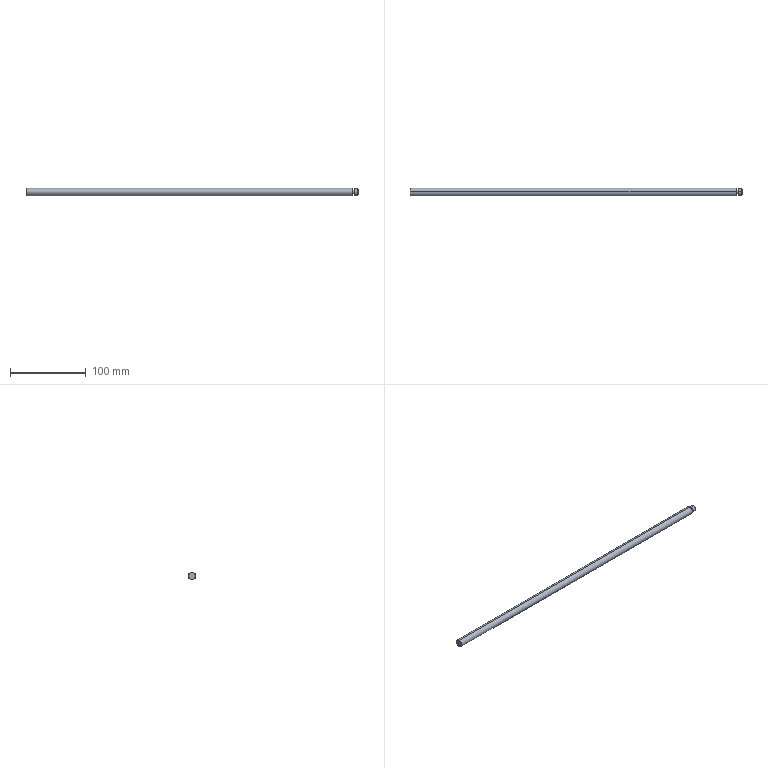Part | SolidWorks | features ICE 2, Chamfer 1, Extrusion 1 | 1 solid | 16 faces | box 437 x 10 x 10 mm | volume 34052 mm3 | cone 6 | cylinder 6 | plane 4 | commonest cylinder face diameters 5 x2 8 x2 10 x2
STEP:
#1=CARTESIAN_POINT('',(215.,0.,-4.5));
#2=VERTEX_POINT('',#1);
#3=CARTESIAN_POINT('',(215.,0.,4.5));
#4=VERTEX_POINT('',#3);
#5=CARTESIAN_POINT('',(215.,0.,0.));
#6=DIRECTION('',(1.,0.,0.));
#7=DIRECTION('',(0.,0.,-1.));
#8=AXIS2_PLACEMENT_3D('',#5,#6,#7);
#9=CIRCLE('',#8,4.5);
#10=EDGE_CURVE('',#2,#4,#9,.T.);
#11=ORIENTED_EDGE('',*,*,#10,.F.);
#12=CARTESIAN_POINT('',(214.5,0.,-5.));
#13=VERTEX_POINT('',#12);
#14=CARTESIAN_POINT('',(215.,0.,-4.5));
#15=DIRECTION('',(-0.7071,0.,-0.7071));
#16=VECTOR('',#15,1000.);
#17=LINE('',#14,#16);
#18=EDGE_CURVE('',#2,#13,#17,.T.);
#19=ORIENTED_EDGE('',*,*,#18,.T.);
#20=CARTESIAN_POINT('',(214.5,0.,5.));
#21=VERTEX_POINT('',#20);
#22=CARTESIAN_POINT('',(214.5,0.,0.));
#23=DIRECTION('',(-1.,0.,0.));
#24=DIRECTION('',(0.,0.,-1.));
#25=AXIS2_PLACEMENT_3D('',#22,#23,#24);
#26=CIRCLE('',#25,5.);
#27=EDGE_CURVE('',#21,#13,#26,.T.);
#28=ORIENTED_EDGE('',*,*,#27,.F.);
#29=CARTESIAN_POINT('',(215.,0.,4.5));
#30=DIRECTION('',(-0.7071,0.,0.7071));
#31=VECTOR('',#30,1000.);
#32=LINE('',#29,#31);
#33=EDGE_CURVE('',#4,#21,#32,.T.);
#34=ORIENTED_EDGE('',*,*,#33,.F.);
#35=EDGE_LOOP('',(#11,#19,#28,#34));
#36=FACE_OUTER_BOUND('',#35,.T.);
#37=CARTESIAN_POINT('',(215.,0.,0.));
#38=DIRECTION('',(-1.,0.,0.));
#39=DIRECTION('',(0.,0.,1.));
#40=AXIS2_PLACEMENT_3D('',#37,#38,#39);
#41=CONICAL_SURFACE('',#40,4.5,0.7854);
#42=ADVANCED_FACE('',(#36),#41,.T.);
#43=CARTESIAN_POINT('',(-215.,0.,4.5));
#44=VERTEX_POINT('',#43);
#45=CARTESIAN_POINT('',(-215.,0.,-4.5));
#46=VERTEX_POINT('',#45);
#47=CARTESIAN_POINT('',(-215.,0.,0.));
#48=DIRECTION('',(-1.,0.,0.));
#49=DIRECTION('',(0.,0.,-1.));
#50=AXIS2_PLACEMENT_3D('',#47,#48,#49);
#51=CIRCLE('',#50,4.5);
#52=EDGE_CURVE('',#44,#46,#51,.T.);
#53=ORIENTED_EDGE('',*,*,#52,.F.);
#54=CARTESIAN_POINT('',(-214.5,0.,5.));
#55=VERTEX_POINT('',#54);
#56=CARTESIAN_POINT('',(-214.5,0.,5.));
#57=DIRECTION('',(0.7071,0.,0.7071));
#58=VECTOR('',#57,1000.);
#59=LINE('',#56,#58);
#60=EDGE_CURVE('',#44,#55,#59,.T.);
#61=ORIENTED_EDGE('',*,*,#60,.T.);
#62=CARTESIAN_POINT('',(-214.5,0.,-5.));
#63=VERTEX_POINT('',#62);
#64=CARTESIAN_POINT('',(-214.5,0.,0.));
#65=DIRECTION('',(1.,0.,0.));
#66=DIRECTION('',(0.,0.,-1.));
#67=AXIS2_PLACEMENT_3D('',#64,#65,#66);
#68=CIRCLE('',#67,5.);
#69=EDGE_CURVE('',#63,#55,#68,.T.);
#70=ORIENTED_EDGE('',*,*,#69,.F.);
#71=CARTESIAN_POINT('',(-214.5,0.,-5.));
#72=DIRECTION('',(0.7071,0.,-0.7071));
#73=VECTOR('',#72,1000.);
#74=LINE('',#71,#73);
#75=EDGE_CURVE('',#46,#63,#74,.T.);
#76=ORIENTED_EDGE('',*,*,#75,.F.);
#77=EDGE_LOOP('',(#53,#61,#70,#76));
#78=FACE_OUTER_BOUND('',#77,.T.);
#79=CARTESIAN_POINT('',(-214.5,0.,0.));
#80=DIRECTION('',(1.,0.,0.));
#81=DIRECTION('',(0.,0.,-1.));
#82=AXIS2_PLACEMENT_3D('',#79,#80,#81);
#83=CONICAL_SURFACE('',#82,5.,0.7854);
#84=ADVANCED_FACE('',(#78),#83,.T.);
#85=CARTESIAN_POINT('',(222.,0.,-3.5));
#86=VERTEX_POINT('',#85);
#87=CARTESIAN_POINT('',(222.,0.,3.5));
#88=VERTEX_POINT('',#87);
#89=CARTESIAN_POINT('',(222.,0.,0.));
#90=DIRECTION('',(1.,0.,0.));
#91=DIRECTION('',(0.,0.,-1.));
#92=AXIS2_PLACEMENT_3D('',#89,#90,#91);
#93=CIRCLE('',#92,3.5);
#94=EDGE_CURVE('',#86,#88,#93,.T.);
#95=ORIENTED_EDGE('',*,*,#94,.F.);
#96=CARTESIAN_POINT('',(221.5,0.,-4.));
#97=VERTEX_POINT('',#96);
#98=CARTESIAN_POINT('',(222.,0.,-3.5));
#99=DIRECTION('',(-0.7071,0.,-0.7071));
#100=VECTOR('',#99,1000.);
#101=LINE('',#98,#100);
#102=EDGE_CURVE('',#86,#97,#101,.T.);
#103=ORIENTED_EDGE('',*,*,#102,.T.);
#104=CARTESIAN_POINT('',(221.5,0.,4.));
#105=VERTEX_POINT('',#104);
#106=CARTESIAN_POINT('',(221.5,0.,0.));
#107=DIRECTION('',(-1.,0.,0.));
#108=DIRECTION('',(0.,0.,-1.));
#109=AXIS2_PLACEMENT_3D('',#106,#107,#108);
#110=CIRCLE('',#109,4.);
#111=EDGE_CURVE('',#105,#97,#110,.T.);
#112=ORIENTED_EDGE('',*,*,#111,.F.);
#113=CARTESIAN_POINT('',(222.,0.,3.5));
#114=DIRECTION('',(-0.7071,0.,0.7071));
#115=VECTOR('',#114,1000.);
#116=LINE('',#113,#115);
#117=EDGE_CURVE('',#88,#105,#116,.T.);
#118=ORIENTED_EDGE('',*,*,#117,.F.);
#119=EDGE_LOOP('',(#95,#103,#112,#118));
#120=FACE_OUTER_BOUND('',#119,.T.);
#121=CARTESIAN_POINT('',(222.,0.,0.));
#122=DIRECTION('',(-1.,0.,0.));
#123=DIRECTION('',(0.,0.,1.));
#124=AXIS2_PLACEMENT_3D('',#121,#122,#123);
#125=CONICAL_SURFACE('',#124,3.5,0.7854);
#126=ADVANCED_FACE('',(#120),#125,.T.);
#127=ORIENTED_EDGE('',*,*,#111,.T.);
#128=CARTESIAN_POINT('',(217.,0.,-4.));
#129=VERTEX_POINT('',#128);
#130=CARTESIAN_POINT('',(222.,0.,-4.));
#131=DIRECTION('',(-1.,0.,0.));
#132=VECTOR('',#131,1000.);
#133=LINE('',#130,#132);
#134=EDGE_CURVE('',#97,#129,#133,.T.);
#135=ORIENTED_EDGE('',*,*,#134,.T.);
#136=CARTESIAN_POINT('',(217.,0.,4.));
#137=VERTEX_POINT('',#136);
#138=CARTESIAN_POINT('',(217.,0.,0.));
#139=DIRECTION('',(1.,0.,0.));
#140=DIRECTION('',(0.,0.,-1.));
#141=AXIS2_PLACEMENT_3D('',#138,#139,#140);
#142=CIRCLE('',#141,4.);
#143=EDGE_CURVE('',#129,#137,#142,.T.);
#144=ORIENTED_EDGE('',*,*,#143,.T.);
#145=CARTESIAN_POINT('',(222.,0.,4.));
#146=DIRECTION('',(-1.,0.,0.));
#147=VECTOR('',#146,1000.);
#148=LINE('',#145,#147);
#149=EDGE_CURVE('',#105,#137,#148,.T.);
#150=ORIENTED_EDGE('',*,*,#149,.F.);
#151=EDGE_LOOP('',(#127,#135,#144,#150));
#152=FACE_OUTER_BOUND('',#151,.T.);
#153=CARTESIAN_POINT('',(222.,0.,0.));
#154=DIRECTION('',(-1.,0.,0.));
#155=DIRECTION('',(0.,0.,1.));
#156=AXIS2_PLACEMENT_3D('',#153,#154,#155);
#157=CYLINDRICAL_SURFACE('',#156,4.);
#158=ADVANCED_FACE('',(#152),#157,.T.);
#159=CARTESIAN_POINT('',(217.,0.,-2.5));
#160=VERTEX_POINT('',#159);
#161=CARTESIAN_POINT('',(217.,0.,2.5));
#162=VERTEX_POINT('',#161);
#163=CARTESIAN_POINT('',(217.,0.,0.));
#164=DIRECTION('',(1.,0.,0.));
#165=DIRECTION('',(0.,0.,-1.));
#166=AXIS2_PLACEMENT_3D('',#163,#164,#165);
#167=CIRCLE('',#166,2.5);
#168=EDGE_CURVE('',#160,#162,#167,.T.);
#169=ORIENTED_EDGE('',*,*,#168,.F.);
#170=CARTESIAN_POINT('',(215.,0.,-2.5));
#171=VERTEX_POINT('',#170);
#172=CARTESIAN_POINT('',(217.,0.,-2.5));
#173=DIRECTION('',(-1.,0.,0.));
#174=VECTOR('',#173,1000.);
#175=LINE('',#172,#174);
#176=EDGE_CURVE('',#160,#171,#175,.T.);
#177=ORIENTED_EDGE('',*,*,#176,.T.);
#178=CARTESIAN_POINT('',(215.,0.,2.5));
#179=VERTEX_POINT('',#178);
#180=CARTESIAN_POINT('',(215.,0.,0.));
#181=DIRECTION('',(1.,0.,0.));
#182=DIRECTION('',(0.,0.,-1.));
#183=AXIS2_PLACEMENT_3D('',#180,#181,#182);
#184=CIRCLE('',#183,2.5);
#185=EDGE_CURVE('',#171,#179,#184,.T.);
#186=ORIENTED_EDGE('',*,*,#185,.T.);
#187=CARTESIAN_POINT('',(217.,0.,2.5));
#188=DIRECTION('',(-1.,0.,0.));
#189=VECTOR('',#188,1000.);
#190=LINE('',#187,#189);
#191=EDGE_CURVE('',#162,#179,#190,.T.);
#192=ORIENTED_EDGE('',*,*,#191,.F.);
#193=EDGE_LOOP('',(#169,#177,#186,#192));
#194=FACE_OUTER_BOUND('',#193,.T.);
#195=CARTESIAN_POINT('',(217.,0.,0.));
#196=DIRECTION('',(-1.,0.,0.));
#197=DIRECTION('',(0.,0.,1.));
#198=AXIS2_PLACEMENT_3D('',#195,#196,#197);
#199=CYLINDRICAL_SURFACE('',#198,2.5);
#200=ADVANCED_FACE('',(#194),#199,.T.);
#201=ORIENTED_EDGE('',*,*,#27,.T.);
#202=CARTESIAN_POINT('',(215.,0.,-5.));
#203=DIRECTION('',(-1.,0.,0.));
#204=VECTOR('',#203,1000.);
#205=LINE('',#202,#204);
#206=EDGE_CURVE('',#13,#63,#205,.T.);
#207=ORIENTED_EDGE('',*,*,#206,.T.);
#208=ORIENTED_EDGE('',*,*,#69,.T.);
#209=CARTESIAN_POINT('',(215.,0.,5.));
#210=DIRECTION('',(-1.,0.,0.));
#211=VECTOR('',#210,1000.);
#212=LINE('',#209,#211);
#213=EDGE_CURVE('',#21,#55,#212,.T.);
#214=ORIENTED_EDGE('',*,*,#213,.F.);
#215=EDGE_LOOP('',(#201,#207,#208,#214));
#216=FACE_OUTER_BOUND('',#215,.T.);
#217=CARTESIAN_POINT('',(215.,0.,0.));
#218=DIRECTION('',(-1.,0.,0.));
#219=DIRECTION('',(0.,0.,1.));
#220=AXIS2_PLACEMENT_3D('',#217,#218,#219);
#221=CYLINDRICAL_SURFACE('',#220,5.);
#222=ADVANCED_FACE('',(#216),#221,.T.);
#223=CARTESIAN_POINT('',(215.,0.,0.));
#224=DIRECTION('',(1.,0.,0.));
#225=DIRECTION('',(0.,0.,-1.));
#226=AXIS2_PLACEMENT_3D('',#223,#224,#225);
#227=CIRCLE('',#226,4.5);
#228=EDGE_CURVE('',#4,#2,#227,.T.);
#229=ORIENTED_EDGE('',*,*,#228,.T.);
#230=ORIENTED_EDGE('',*,*,#10,.T.);
#231=EDGE_LOOP('',(#229,#230));
#232=FACE_OUTER_BOUND('',#231,.T.);
#233=CARTESIAN_POINT('',(215.,0.,0.));
#234=DIRECTION('',(1.,0.,0.));
#235=DIRECTION('',(0.,0.,-1.));
#236=AXIS2_PLACEMENT_3D('',#233,#234,#235);
#237=CIRCLE('',#236,2.5);
#238=EDGE_CURVE('',#179,#171,#237,.T.);
#239=ORIENTED_EDGE('',*,*,#238,.F.);
#240=ORIENTED_EDGE('',*,*,#185,.F.);
#241=EDGE_LOOP('',(#239,#240));
#242=FACE_BOUND('',#241,.T.);
#243=CARTESIAN_POINT('',(215.,0.,0.));
#244=DIRECTION('',(1.,0.,0.));
#245=DIRECTION('',(0.,0.,-1.));
#246=AXIS2_PLACEMENT_3D('',#243,#244,#245);
#247=PLANE('',#246);
#248=ADVANCED_FACE('',(#232,#242),#247,.T.);
#249=ORIENTED_EDGE('',*,*,#206,.F.);
#250=CARTESIAN_POINT('',(214.5,0.,0.));
#251=DIRECTION('',(-1.,0.,0.));
#252=DIRECTION('',(0.,0.,-1.));
#253=AXIS2_PLACEMENT_3D('',#250,#251,#252);
#254=CIRCLE('',#253,5.);
#255=EDGE_CURVE('',#13,#21,#254,.T.);
#256=ORIENTED_EDGE('',*,*,#255,.T.);
#257=ORIENTED_EDGE('',*,*,#213,.T.);
#258=CARTESIAN_POINT('',(-214.5,0.,0.));
#259=DIRECTION('',(1.,0.,0.));
#260=DIRECTION('',(0.,0.,-1.));
#261=AXIS2_PLACEMENT_3D('',#258,#259,#260);
#262=CIRCLE('',#261,5.);
#263=EDGE_CURVE('',#55,#63,#262,.T.);
#264=ORIENTED_EDGE('',*,*,#263,.T.);
#265=EDGE_LOOP('',(#249,#256,#257,#264));
#266=FACE_OUTER_BOUND('',#265,.T.);
#267=CARTESIAN_POINT('',(215.,0.,0.));
#268=DIRECTION('',(-1.,0.,0.));
#269=DIRECTION('',(0.,0.,1.));
#270=AXIS2_PLACEMENT_3D('',#267,#268,#269);
#271=CYLINDRICAL_SURFACE('',#270,5.);
#272=ADVANCED_FACE('',(#266),#271,.T.);
#273=CARTESIAN_POINT('',(-215.,0.,0.));
#274=DIRECTION('',(-1.,0.,0.));
#275=DIRECTION('',(0.,0.,-1.));
#276=AXIS2_PLACEMENT_3D('',#273,#274,#275);
#277=CIRCLE('',#276,4.5);
#278=EDGE_CURVE('',#46,#44,#277,.T.);
#279=ORIENTED_EDGE('',*,*,#278,.T.);
#280=ORIENTED_EDGE('',*,*,#52,.T.);
#281=EDGE_LOOP('',(#279,#280));
#282=FACE_OUTER_BOUND('',#281,.T.);
#283=CARTESIAN_POINT('',(-215.,0.,0.));
#284=DIRECTION('',(1.,0.,0.));
#285=DIRECTION('',(0.,0.,-1.));
#286=AXIS2_PLACEMENT_3D('',#283,#284,#285);
#287=PLANE('',#286);
#288=ADVANCED_FACE('',(#282),#287,.F.);
#289=ORIENTED_EDGE('',*,*,#176,.F.);
#290=CARTESIAN_POINT('',(217.,0.,0.));
#291=DIRECTION('',(1.,0.,0.));
#292=DIRECTION('',(0.,0.,-1.));
#293=AXIS2_PLACEMENT_3D('',#290,#291,#292);
#294=CIRCLE('',#293,2.5);
#295=EDGE_CURVE('',#162,#160,#294,.T.);
#296=ORIENTED_EDGE('',*,*,#295,.F.);
#297=ORIENTED_EDGE('',*,*,#191,.T.);
#298=ORIENTED_EDGE('',*,*,#238,.T.);
#299=EDGE_LOOP('',(#289,#296,#297,#298));
#300=FACE_OUTER_BOUND('',#299,.T.);
#301=CARTESIAN_POINT('',(217.,0.,0.));
#302=DIRECTION('',(-1.,0.,0.));
#303=DIRECTION('',(0.,0.,1.));
#304=AXIS2_PLACEMENT_3D('',#301,#302,#303);
#305=CYLINDRICAL_SURFACE('',#304,2.5);
#306=ADVANCED_FACE('',(#300),#305,.T.);
#307=CARTESIAN_POINT('',(217.,0.,0.));
#308=DIRECTION('',(1.,0.,0.));
#309=DIRECTION('',(0.,0.,-1.));
#310=AXIS2_PLACEMENT_3D('',#307,#308,#309);
#311=CIRCLE('',#310,4.);
#312=EDGE_CURVE('',#137,#129,#311,.T.);
#313=ORIENTED_EDGE('',*,*,#312,.F.);
#314=ORIENTED_EDGE('',*,*,#143,.F.);
#315=EDGE_LOOP('',(#313,#314));
#316=FACE_OUTER_BOUND('',#315,.T.);
#317=ORIENTED_EDGE('',*,*,#295,.T.);
#318=ORIENTED_EDGE('',*,*,#168,.T.);
#319=EDGE_LOOP('',(#317,#318));
#320=FACE_BOUND('',#319,.T.);
#321=CARTESIAN_POINT('',(217.,0.,0.));
#322=DIRECTION('',(1.,0.,0.));
#323=DIRECTION('',(0.,0.,-1.));
#324=AXIS2_PLACEMENT_3D('',#321,#322,#323);
#325=PLANE('',#324);
#326=ADVANCED_FACE('',(#316,#320),#325,.F.);
#327=ORIENTED_EDGE('',*,*,#134,.F.);
#328=CARTESIAN_POINT('',(221.5,0.,0.));
#329=DIRECTION('',(-1.,0.,0.));
#330=DIRECTION('',(0.,0.,-1.));
#331=AXIS2_PLACEMENT_3D('',#328,#329,#330);
#332=CIRCLE('',#331,4.);
#333=EDGE_CURVE('',#97,#105,#332,.T.);
#334=ORIENTED_EDGE('',*,*,#333,.T.);
#335=ORIENTED_EDGE('',*,*,#149,.T.);
#336=ORIENTED_EDGE('',*,*,#312,.T.);
#337=EDGE_LOOP('',(#327,#334,#335,#336));
#338=FACE_OUTER_BOUND('',#337,.T.);
#339=CARTESIAN_POINT('',(222.,0.,0.));
#340=DIRECTION('',(-1.,0.,0.));
#341=DIRECTION('',(0.,0.,1.));
#342=AXIS2_PLACEMENT_3D('',#339,#340,#341);
#343=CYLINDRICAL_SURFACE('',#342,4.);
#344=ADVANCED_FACE('',(#338),#343,.T.);
#345=CARTESIAN_POINT('',(222.,0.,0.));
#346=DIRECTION('',(1.,0.,0.));
#347=DIRECTION('',(0.,0.,-1.));
#348=AXIS2_PLACEMENT_3D('',#345,#346,#347);
#349=CIRCLE('',#348,3.5);
#350=EDGE_CURVE('',#88,#86,#349,.T.);
#351=ORIENTED_EDGE('',*,*,#350,.T.);
#352=ORIENTED_EDGE('',*,*,#94,.T.);
#353=EDGE_LOOP('',(#351,#352));
#354=FACE_OUTER_BOUND('',#353,.T.);
#355=CARTESIAN_POINT('',(222.,0.,0.));
#356=DIRECTION('',(1.,0.,0.));
#357=DIRECTION('',(0.,0.,-1.));
#358=AXIS2_PLACEMENT_3D('',#355,#356,#357);
#359=PLANE('',#358);
#360=ADVANCED_FACE('',(#354),#359,.T.);
#361=ORIENTED_EDGE('',*,*,#102,.F.);
#362=ORIENTED_EDGE('',*,*,#350,.F.);
#363=ORIENTED_EDGE('',*,*,#117,.T.);
#364=ORIENTED_EDGE('',*,*,#333,.F.);
#365=EDGE_LOOP('',(#361,#362,#363,#364));
#366=FACE_OUTER_BOUND('',#365,.T.);
#367=CARTESIAN_POINT('',(222.,0.,0.));
#368=DIRECTION('',(-1.,0.,0.));
#369=DIRECTION('',(0.,0.,1.));
#370=AXIS2_PLACEMENT_3D('',#367,#368,#369);
#371=CONICAL_SURFACE('',#370,3.5,0.7854);
#372=ADVANCED_FACE('',(#366),#371,.T.);
#373=ORIENTED_EDGE('',*,*,#60,.F.);
#374=ORIENTED_EDGE('',*,*,#278,.F.);
#375=ORIENTED_EDGE('',*,*,#75,.T.);
#376=ORIENTED_EDGE('',*,*,#263,.F.);
#377=EDGE_LOOP('',(#373,#374,#375,#376));
#378=FACE_OUTER_BOUND('',#377,.T.);
#379=CARTESIAN_POINT('',(-214.5,0.,0.));
#380=DIRECTION('',(1.,0.,0.));
#381=DIRECTION('',(0.,0.,-1.));
#382=AXIS2_PLACEMENT_3D('',#379,#380,#381);
#383=CONICAL_SURFACE('',#382,5.,0.7854);
#384=ADVANCED_FACE('',(#378),#383,.T.);
#385=ORIENTED_EDGE('',*,*,#18,.F.);
#386=ORIENTED_EDGE('',*,*,#228,.F.);
#387=ORIENTED_EDGE('',*,*,#33,.T.);
#388=ORIENTED_EDGE('',*,*,#255,.F.);
#389=EDGE_LOOP('',(#385,#386,#387,#388));
#390=FACE_OUTER_BOUND('',#389,.T.);
#391=CARTESIAN_POINT('',(215.,0.,0.));
#392=DIRECTION('',(-1.,0.,0.));
#393=DIRECTION('',(0.,0.,1.));
#394=AXIS2_PLACEMENT_3D('',#391,#392,#393);
#395=CONICAL_SURFACE('',#394,4.5,0.7854);
#396=ADVANCED_FACE('',(#390),#395,.T.);
#397=CLOSED_SHELL('',(#42,#84,#126,#158,#200,#222,#248,#272,#288,#306,#326,#344,#360,#372,#384,#396));
#398=MANIFOLD_SOLID_BREP('',#397);
#399=CARTESIAN_POINT('',(0.,0.,0.));
#400=DIRECTION('',(0.,0.,1.));
#401=DIRECTION('',(1.,0.,0.));
#402=AXIS2_PLACEMENT_3D('',#399,#400,#401);
#403=(LENGTH_UNIT()NAMED_UNIT(*)SI_UNIT(.MILLI.,.METRE.));
#404=UNCERTAINTY_MEASURE_WITH_UNIT(LENGTH_MEASURE(0.00001),#403,'','');
#405=(NAMED_UNIT(*)PLANE_ANGLE_UNIT()SI_UNIT($,.RADIAN.));
#406=(NAMED_UNIT(*)SI_UNIT($,.STERADIAN.)SOLID_ANGLE_UNIT());
#407=(GEOMETRIC_REPRESENTATION_CONTEXT(3)GLOBAL_UNCERTAINTY_ASSIGNED_CONTEXT((#404))GLOBAL_UNIT_ASSIGNED_CONTEXT((#403,#405,#406))REPRESENTATION_CONTEXT('',''));
#408=ADVANCED_BREP_SHAPE_REPRESENTATION('',(#398,#402),#407);